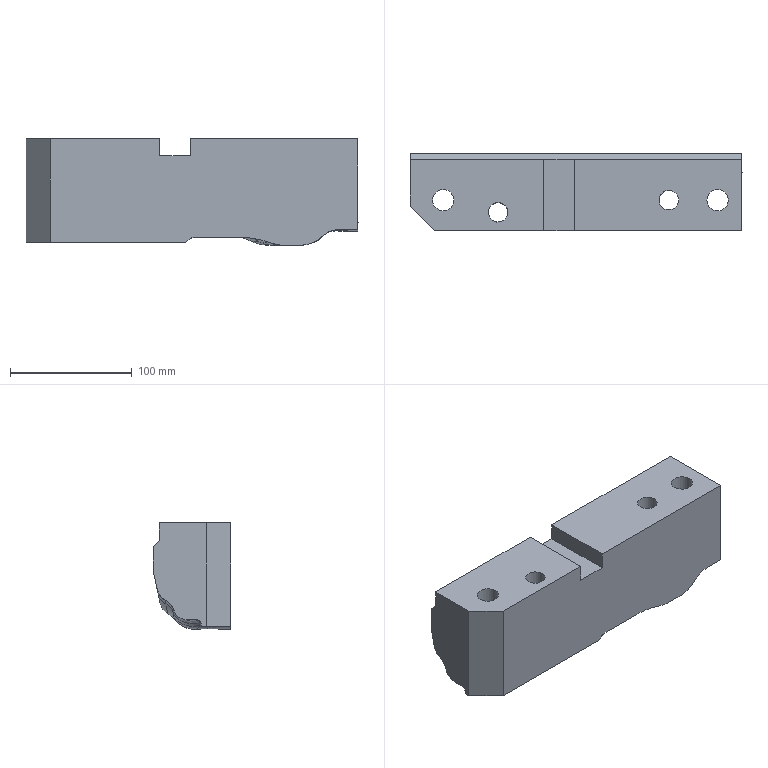Part | NX | features solid 2 | 1 solid | 80 faces | box 272.184 x 63.479 x 88.007 mm | volume 1143991 mm3 | spline 62 | plane 12 | cylinder 6 | commonest cylinder face diameters 16 x2 17.5 x2 25.5 x2